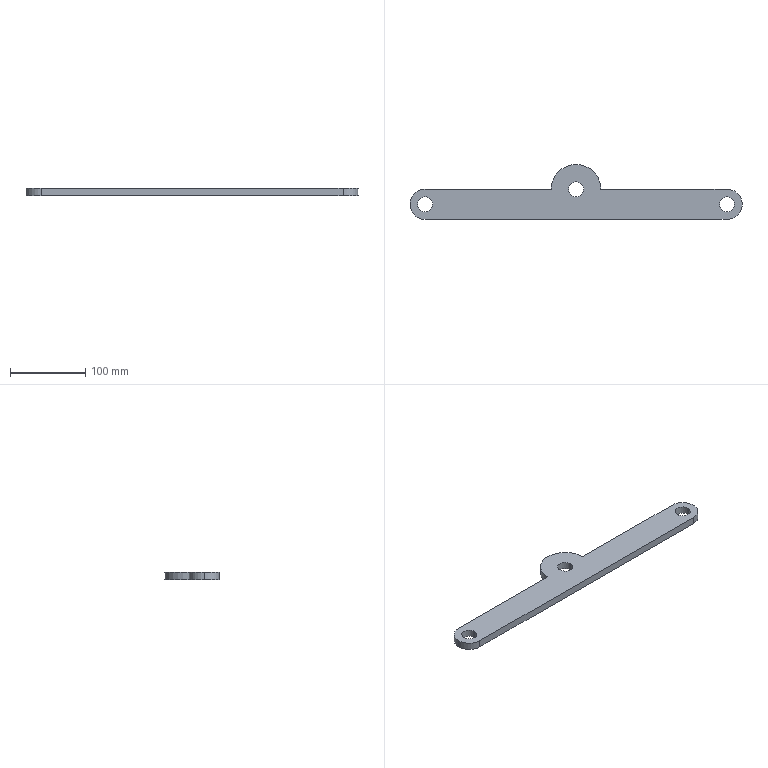Part | SolidWorks | features ICE 3, Extrusion 1 | 1 solid | 15 faces | box 440 x 72.879 x 10 mm | volume 180122 mm3 | cylinder 10 | plane 5 | commonest cylinder face diameters 20 x6 40 x3 65.758 x1
STEP:
#1=CARTESIAN_POINT('',(-10.,20.,0.));
#2=VERTEX_POINT('',#1);
#3=CARTESIAN_POINT('',(10.,20.,0.));
#4=VERTEX_POINT('',#3);
#5=CARTESIAN_POINT('',(0.,20.,0.));
#6=DIRECTION('',(0.,0.,1.));
#7=DIRECTION('',(1.,0.,0.));
#8=AXIS2_PLACEMENT_3D('',#5,#6,#7);
#9=CIRCLE('',#8,10.);
#10=EDGE_CURVE('',#2,#4,#9,.T.);
#11=ORIENTED_EDGE('',*,*,#10,.F.);
#12=CARTESIAN_POINT('',(-10.,20.,10.));
#13=VERTEX_POINT('',#12);
#14=CARTESIAN_POINT('',(-10.,20.,0.));
#15=DIRECTION('',(0.,0.,1.));
#16=VECTOR('',#15,1000.);
#17=LINE('',#14,#16);
#18=EDGE_CURVE('',#2,#13,#17,.T.);
#19=ORIENTED_EDGE('',*,*,#18,.T.);
#20=CARTESIAN_POINT('',(10.,20.,10.));
#21=VERTEX_POINT('',#20);
#22=CARTESIAN_POINT('',(0.,20.,10.));
#23=DIRECTION('',(0.,0.,1.));
#24=DIRECTION('',(1.,0.,0.));
#25=AXIS2_PLACEMENT_3D('',#22,#23,#24);
#26=CIRCLE('',#25,10.);
#27=EDGE_CURVE('',#13,#21,#26,.T.);
#28=ORIENTED_EDGE('',*,*,#27,.T.);
#29=CARTESIAN_POINT('',(10.,20.,0.));
#30=DIRECTION('',(0.,0.,1.));
#31=VECTOR('',#30,1000.);
#32=LINE('',#29,#31);
#33=EDGE_CURVE('',#4,#21,#32,.T.);
#34=ORIENTED_EDGE('',*,*,#33,.F.);
#35=EDGE_LOOP('',(#11,#19,#28,#34));
#36=FACE_OUTER_BOUND('',#35,.T.);
#37=CARTESIAN_POINT('',(0.,20.,0.));
#38=DIRECTION('',(0.,0.,1.));
#39=DIRECTION('',(1.,0.,0.));
#40=AXIS2_PLACEMENT_3D('',#37,#38,#39);
#41=CYLINDRICAL_SURFACE('',#40,10.);
#42=ADVANCED_FACE('',(#36),#41,.F.);
#43=CARTESIAN_POINT('',(-210.,0.,0.));
#44=VERTEX_POINT('',#43);
#45=CARTESIAN_POINT('',(-190.,0.,0.));
#46=VERTEX_POINT('',#45);
#47=CARTESIAN_POINT('',(-200.,0.,0.));
#48=DIRECTION('',(0.,0.,1.));
#49=DIRECTION('',(1.,0.,0.));
#50=AXIS2_PLACEMENT_3D('',#47,#48,#49);
#51=CIRCLE('',#50,10.);
#52=EDGE_CURVE('',#44,#46,#51,.T.);
#53=ORIENTED_EDGE('',*,*,#52,.F.);
#54=CARTESIAN_POINT('',(-210.,0.,10.));
#55=VERTEX_POINT('',#54);
#56=CARTESIAN_POINT('',(-210.,0.,0.));
#57=DIRECTION('',(0.,0.,1.));
#58=VECTOR('',#57,1000.);
#59=LINE('',#56,#58);
#60=EDGE_CURVE('',#44,#55,#59,.T.);
#61=ORIENTED_EDGE('',*,*,#60,.T.);
#62=CARTESIAN_POINT('',(-190.,0.,10.));
#63=VERTEX_POINT('',#62);
#64=CARTESIAN_POINT('',(-200.,0.,10.));
#65=DIRECTION('',(0.,0.,1.));
#66=DIRECTION('',(1.,0.,0.));
#67=AXIS2_PLACEMENT_3D('',#64,#65,#66);
#68=CIRCLE('',#67,10.);
#69=EDGE_CURVE('',#55,#63,#68,.T.);
#70=ORIENTED_EDGE('',*,*,#69,.T.);
#71=CARTESIAN_POINT('',(-190.,0.,0.));
#72=DIRECTION('',(0.,0.,1.));
#73=VECTOR('',#72,1000.);
#74=LINE('',#71,#73);
#75=EDGE_CURVE('',#46,#63,#74,.T.);
#76=ORIENTED_EDGE('',*,*,#75,.F.);
#77=EDGE_LOOP('',(#53,#61,#70,#76));
#78=FACE_OUTER_BOUND('',#77,.T.);
#79=CARTESIAN_POINT('',(-200.,0.,0.));
#80=DIRECTION('',(0.,0.,1.));
#81=DIRECTION('',(1.,0.,0.));
#82=AXIS2_PLACEMENT_3D('',#79,#80,#81);
#83=CYLINDRICAL_SURFACE('',#82,10.);
#84=ADVANCED_FACE('',(#78),#83,.F.);
#85=CARTESIAN_POINT('',(190.,0.,0.));
#86=VERTEX_POINT('',#85);
#87=CARTESIAN_POINT('',(210.,0.,0.));
#88=VERTEX_POINT('',#87);
#89=CARTESIAN_POINT('',(200.,0.,0.));
#90=DIRECTION('',(0.,0.,1.));
#91=DIRECTION('',(1.,0.,0.));
#92=AXIS2_PLACEMENT_3D('',#89,#90,#91);
#93=CIRCLE('',#92,10.);
#94=EDGE_CURVE('',#86,#88,#93,.T.);
#95=ORIENTED_EDGE('',*,*,#94,.F.);
#96=CARTESIAN_POINT('',(190.,0.,10.));
#97=VERTEX_POINT('',#96);
#98=CARTESIAN_POINT('',(190.,0.,0.));
#99=DIRECTION('',(0.,0.,1.));
#100=VECTOR('',#99,1000.);
#101=LINE('',#98,#100);
#102=EDGE_CURVE('',#86,#97,#101,.T.);
#103=ORIENTED_EDGE('',*,*,#102,.T.);
#104=CARTESIAN_POINT('',(210.,0.,10.));
#105=VERTEX_POINT('',#104);
#106=CARTESIAN_POINT('',(200.,0.,10.));
#107=DIRECTION('',(0.,0.,1.));
#108=DIRECTION('',(1.,0.,0.));
#109=AXIS2_PLACEMENT_3D('',#106,#107,#108);
#110=CIRCLE('',#109,10.);
#111=EDGE_CURVE('',#97,#105,#110,.T.);
#112=ORIENTED_EDGE('',*,*,#111,.T.);
#113=CARTESIAN_POINT('',(210.,0.,0.));
#114=DIRECTION('',(0.,0.,1.));
#115=VECTOR('',#114,1000.);
#116=LINE('',#113,#115);
#117=EDGE_CURVE('',#88,#105,#116,.T.);
#118=ORIENTED_EDGE('',*,*,#117,.F.);
#119=EDGE_LOOP('',(#95,#103,#112,#118));
#120=FACE_OUTER_BOUND('',#119,.T.);
#121=CARTESIAN_POINT('',(200.,0.,0.));
#122=DIRECTION('',(0.,0.,1.));
#123=DIRECTION('',(1.,0.,0.));
#124=AXIS2_PLACEMENT_3D('',#121,#122,#123);
#125=CYLINDRICAL_SURFACE('',#124,10.);
#126=ADVANCED_FACE('',(#120),#125,.F.);
#127=CARTESIAN_POINT('',(-220.,0.,10.));
#128=VERTEX_POINT('',#127);
#129=CARTESIAN_POINT('',(-200.,-20.,10.));
#130=VERTEX_POINT('',#129);
#131=CARTESIAN_POINT('',(-200.,0.,10.));
#132=DIRECTION('',(0.,0.,1.));
#133=DIRECTION('',(1.,0.,0.));
#134=AXIS2_PLACEMENT_3D('',#131,#132,#133);
#135=CIRCLE('',#134,20.);
#136=EDGE_CURVE('',#128,#130,#135,.T.);
#137=ORIENTED_EDGE('',*,*,#136,.F.);
#138=CARTESIAN_POINT('',(-220.,0.,0.));
#139=VERTEX_POINT('',#138);
#140=CARTESIAN_POINT('',(-220.,0.,10.));
#141=DIRECTION('',(0.,0.,-1.));
#142=VECTOR('',#141,1000.);
#143=LINE('',#140,#142);
#144=EDGE_CURVE('',#128,#139,#143,.T.);
#145=ORIENTED_EDGE('',*,*,#144,.T.);
#146=CARTESIAN_POINT('',(-200.,-20.,0.));
#147=VERTEX_POINT('',#146);
#148=CARTESIAN_POINT('',(-200.,0.,0.));
#149=DIRECTION('',(0.,0.,1.));
#150=DIRECTION('',(1.,0.,0.));
#151=AXIS2_PLACEMENT_3D('',#148,#149,#150);
#152=CIRCLE('',#151,20.);
#153=EDGE_CURVE('',#139,#147,#152,.T.);
#154=ORIENTED_EDGE('',*,*,#153,.T.);
#155=CARTESIAN_POINT('',(-200.,-20.,10.));
#156=DIRECTION('',(0.,0.,-1.));
#157=VECTOR('',#156,1000.);
#158=LINE('',#155,#157);
#159=EDGE_CURVE('',#130,#147,#158,.T.);
#160=ORIENTED_EDGE('',*,*,#159,.F.);
#161=EDGE_LOOP('',(#137,#145,#154,#160));
#162=FACE_OUTER_BOUND('',#161,.T.);
#163=CARTESIAN_POINT('',(-200.,0.,10.));
#164=DIRECTION('',(0.,0.,-1.));
#165=DIRECTION('',(-1.,0.,0.));
#166=AXIS2_PLACEMENT_3D('',#163,#164,#165);
#167=CYLINDRICAL_SURFACE('',#166,20.);
#168=ADVANCED_FACE('',(#162),#167,.T.);
#169=CARTESIAN_POINT('',(200.,20.,0.));
#170=VERTEX_POINT('',#169);
#171=CARTESIAN_POINT('',(32.879,20.,0.));
#172=VERTEX_POINT('',#171);
#173=CARTESIAN_POINT('',(-200.,20.,0.));
#174=DIRECTION('',(-1.,0.,0.));
#175=VECTOR('',#174,1000.);
#176=LINE('',#173,#175);
#177=EDGE_CURVE('',#170,#172,#176,.T.);
#178=ORIENTED_EDGE('',*,*,#177,.T.);
#179=CARTESIAN_POINT('',(32.879,20.,10.));
#180=VERTEX_POINT('',#179);
#181=CARTESIAN_POINT('',(32.879,20.,-92.996));
#182=DIRECTION('',(0.,0.,1.));
#183=VECTOR('',#182,1000.);
#184=LINE('',#181,#183);
#185=EDGE_CURVE('',#172,#180,#184,.T.);
#186=ORIENTED_EDGE('',*,*,#185,.T.);
#187=CARTESIAN_POINT('',(200.,20.,10.));
#188=VERTEX_POINT('',#187);
#189=CARTESIAN_POINT('',(-200.,20.,10.));
#190=DIRECTION('',(-1.,0.,0.));
#191=VECTOR('',#190,1000.);
#192=LINE('',#189,#191);
#193=EDGE_CURVE('',#188,#180,#192,.T.);
#194=ORIENTED_EDGE('',*,*,#193,.F.);
#195=CARTESIAN_POINT('',(200.,20.,10.));
#196=DIRECTION('',(0.,0.,-1.));
#197=VECTOR('',#196,1000.);
#198=LINE('',#195,#197);
#199=EDGE_CURVE('',#188,#170,#198,.T.);
#200=ORIENTED_EDGE('',*,*,#199,.T.);
#201=EDGE_LOOP('',(#178,#186,#194,#200));
#202=FACE_OUTER_BOUND('',#201,.T.);
#203=CARTESIAN_POINT('',(-200.,20.,10.));
#204=DIRECTION('',(0.,-1.,0.));
#205=DIRECTION('',(1.,0.,0.));
#206=AXIS2_PLACEMENT_3D('',#203,#204,#205);
#207=PLANE('',#206);
#208=ADVANCED_FACE('',(#202),#207,.F.);
#209=ORIENTED_EDGE('',*,*,#144,.F.);
#210=CARTESIAN_POINT('',(-200.,20.,10.));
#211=VERTEX_POINT('',#210);
#212=CARTESIAN_POINT('',(-200.,0.,10.));
#213=DIRECTION('',(0.,0.,1.));
#214=DIRECTION('',(1.,0.,0.));
#215=AXIS2_PLACEMENT_3D('',#212,#213,#214);
#216=CIRCLE('',#215,20.);
#217=EDGE_CURVE('',#211,#128,#216,.T.);
#218=ORIENTED_EDGE('',*,*,#217,.F.);
#219=CARTESIAN_POINT('',(-200.,20.,0.));
#220=VERTEX_POINT('',#219);
#221=CARTESIAN_POINT('',(-200.,20.,10.));
#222=DIRECTION('',(0.,0.,-1.));
#223=VECTOR('',#222,1000.);
#224=LINE('',#221,#223);
#225=EDGE_CURVE('',#211,#220,#224,.T.);
#226=ORIENTED_EDGE('',*,*,#225,.T.);
#227=CARTESIAN_POINT('',(-200.,0.,0.));
#228=DIRECTION('',(0.,0.,1.));
#229=DIRECTION('',(1.,0.,0.));
#230=AXIS2_PLACEMENT_3D('',#227,#228,#229);
#231=CIRCLE('',#230,20.);
#232=EDGE_CURVE('',#220,#139,#231,.T.);
#233=ORIENTED_EDGE('',*,*,#232,.T.);
#234=EDGE_LOOP('',(#209,#218,#226,#233));
#235=FACE_OUTER_BOUND('',#234,.T.);
#236=CARTESIAN_POINT('',(-200.,0.,10.));
#237=DIRECTION('',(0.,0.,-1.));
#238=DIRECTION('',(-1.,0.,0.));
#239=AXIS2_PLACEMENT_3D('',#236,#237,#238);
#240=CYLINDRICAL_SURFACE('',#239,20.);
#241=ADVANCED_FACE('',(#235),#240,.T.);
#242=CARTESIAN_POINT('',(200.,-20.,0.));
#243=VERTEX_POINT('',#242);
#244=CARTESIAN_POINT('',(-200.,-20.,0.));
#245=DIRECTION('',(1.,0.,0.));
#246=VECTOR('',#245,1000.);
#247=LINE('',#244,#246);
#248=EDGE_CURVE('',#147,#243,#247,.T.);
#249=ORIENTED_EDGE('',*,*,#248,.T.);
#250=CARTESIAN_POINT('',(200.,-20.,10.));
#251=VERTEX_POINT('',#250);
#252=CARTESIAN_POINT('',(200.,-20.,10.));
#253=DIRECTION('',(0.,0.,-1.));
#254=VECTOR('',#253,1000.);
#255=LINE('',#252,#254);
#256=EDGE_CURVE('',#251,#243,#255,.T.);
#257=ORIENTED_EDGE('',*,*,#256,.F.);
#258=CARTESIAN_POINT('',(-200.,-20.,10.));
#259=DIRECTION('',(1.,0.,0.));
#260=VECTOR('',#259,1000.);
#261=LINE('',#258,#260);
#262=EDGE_CURVE('',#130,#251,#261,.T.);
#263=ORIENTED_EDGE('',*,*,#262,.F.);
#264=ORIENTED_EDGE('',*,*,#159,.T.);
#265=EDGE_LOOP('',(#249,#257,#263,#264));
#266=FACE_OUTER_BOUND('',#265,.T.);
#267=CARTESIAN_POINT('',(-200.,-20.,10.));
#268=DIRECTION('',(0.,1.,0.));
#269=DIRECTION('',(0.,0.,1.));
#270=AXIS2_PLACEMENT_3D('',#267,#268,#269);
#271=PLANE('',#270);
#272=ADVANCED_FACE('',(#266),#271,.F.);
#273=CARTESIAN_POINT('',(200.,0.,0.));
#274=DIRECTION('',(0.,0.,1.));
#275=DIRECTION('',(1.,0.,0.));
#276=AXIS2_PLACEMENT_3D('',#273,#274,#275);
#277=CIRCLE('',#276,20.);
#278=EDGE_CURVE('',#243,#170,#277,.T.);
#279=ORIENTED_EDGE('',*,*,#278,.T.);
#280=ORIENTED_EDGE('',*,*,#199,.F.);
#281=CARTESIAN_POINT('',(200.,0.,10.));
#282=DIRECTION('',(0.,0.,1.));
#283=DIRECTION('',(1.,0.,0.));
#284=AXIS2_PLACEMENT_3D('',#281,#282,#283);
#285=CIRCLE('',#284,20.);
#286=EDGE_CURVE('',#251,#188,#285,.T.);
#287=ORIENTED_EDGE('',*,*,#286,.F.);
#288=ORIENTED_EDGE('',*,*,#256,.T.);
#289=EDGE_LOOP('',(#279,#280,#287,#288));
#290=FACE_OUTER_BOUND('',#289,.T.);
#291=CARTESIAN_POINT('',(200.,0.,10.));
#292=DIRECTION('',(0.,0.,-1.));
#293=DIRECTION('',(-1.,0.,0.));
#294=AXIS2_PLACEMENT_3D('',#291,#292,#293);
#295=CYLINDRICAL_SURFACE('',#294,20.);
#296=ADVANCED_FACE('',(#290),#295,.T.);
#297=CARTESIAN_POINT('',(-32.879,20.,10.));
#298=VERTEX_POINT('',#297);
#299=CARTESIAN_POINT('',(-200.,20.,10.));
#300=DIRECTION('',(-1.,0.,0.));
#301=VECTOR('',#300,1000.);
#302=LINE('',#299,#301);
#303=EDGE_CURVE('',#298,#211,#302,.T.);
#304=ORIENTED_EDGE('',*,*,#303,.F.);
#305=CARTESIAN_POINT('',(-32.879,20.,0.));
#306=VERTEX_POINT('',#305);
#307=CARTESIAN_POINT('',(-32.879,20.,-92.996));
#308=DIRECTION('',(0.,0.,-1.));
#309=VECTOR('',#308,1000.);
#310=LINE('',#307,#309);
#311=EDGE_CURVE('',#298,#306,#310,.T.);
#312=ORIENTED_EDGE('',*,*,#311,.T.);
#313=CARTESIAN_POINT('',(-200.,20.,0.));
#314=DIRECTION('',(-1.,0.,0.));
#315=VECTOR('',#314,1000.);
#316=LINE('',#313,#315);
#317=EDGE_CURVE('',#306,#220,#316,.T.);
#318=ORIENTED_EDGE('',*,*,#317,.T.);
#319=ORIENTED_EDGE('',*,*,#225,.F.);
#320=EDGE_LOOP('',(#304,#312,#318,#319));
#321=FACE_OUTER_BOUND('',#320,.T.);
#322=CARTESIAN_POINT('',(-200.,20.,10.));
#323=DIRECTION('',(0.,-1.,0.));
#324=DIRECTION('',(1.,0.,0.));
#325=AXIS2_PLACEMENT_3D('',#322,#323,#324);
#326=PLANE('',#325);
#327=ADVANCED_FACE('',(#321),#326,.F.);
#328=CARTESIAN_POINT('',(0.,20.,10.));
#329=DIRECTION('',(0.,0.,1.));
#330=DIRECTION('',(1.,0.,0.));
#331=AXIS2_PLACEMENT_3D('',#328,#329,#330);
#332=CIRCLE('',#331,10.);
#333=EDGE_CURVE('',#21,#13,#332,.T.);
#334=ORIENTED_EDGE('',*,*,#333,.F.);
#335=ORIENTED_EDGE('',*,*,#27,.F.);
#336=EDGE_LOOP('',(#334,#335));
#337=FACE_BOUND('',#336,.T.);
#338=ORIENTED_EDGE('',*,*,#193,.T.);
#339=CARTESIAN_POINT('',(0.,20.,10.));
#340=DIRECTION('',(0.,0.,1.));
#341=DIRECTION('',(1.,0.,0.));
#342=AXIS2_PLACEMENT_3D('',#339,#340,#341);
#343=CIRCLE('',#342,32.879);
#344=EDGE_CURVE('',#180,#298,#343,.T.);
#345=ORIENTED_EDGE('',*,*,#344,.T.);
#346=ORIENTED_EDGE('',*,*,#303,.T.);
#347=ORIENTED_EDGE('',*,*,#217,.T.);
#348=ORIENTED_EDGE('',*,*,#136,.T.);
#349=ORIENTED_EDGE('',*,*,#262,.T.);
#350=ORIENTED_EDGE('',*,*,#286,.T.);
#351=EDGE_LOOP('',(#338,#345,#346,#347,#348,#349,#350));
#352=FACE_OUTER_BOUND('',#351,.T.);
#353=CARTESIAN_POINT('',(-200.,0.,10.));
#354=DIRECTION('',(0.,0.,1.));
#355=DIRECTION('',(1.,0.,0.));
#356=AXIS2_PLACEMENT_3D('',#353,#354,#355);
#357=CIRCLE('',#356,10.);
#358=EDGE_CURVE('',#63,#55,#357,.T.);
#359=ORIENTED_EDGE('',*,*,#358,.F.);
#360=ORIENTED_EDGE('',*,*,#69,.F.);
#361=EDGE_LOOP('',(#359,#360));
#362=FACE_BOUND('',#361,.T.);
#363=CARTESIAN_POINT('',(200.,0.,10.));
#364=DIRECTION('',(0.,0.,1.));
#365=DIRECTION('',(1.,0.,0.));
#366=AXIS2_PLACEMENT_3D('',#363,#364,#365);
#367=CIRCLE('',#366,10.);
#368=EDGE_CURVE('',#105,#97,#367,.T.);
#369=ORIENTED_EDGE('',*,*,#368,.F.);
#370=ORIENTED_EDGE('',*,*,#111,.F.);
#371=EDGE_LOOP('',(#369,#370));
#372=FACE_BOUND('',#371,.T.);
#373=CARTESIAN_POINT('',(-200.,0.,10.));
#374=DIRECTION('',(0.,0.,1.));
#375=DIRECTION('',(1.,0.,0.));
#376=AXIS2_PLACEMENT_3D('',#373,#374,#375);
#377=PLANE('',#376);
#378=ADVANCED_FACE('',(#337,#352,#362,#372),#377,.T.);
#379=CARTESIAN_POINT('',(0.,20.,0.));
#380=DIRECTION('',(0.,0.,1.));
#381=DIRECTION('',(1.,0.,0.));
#382=AXIS2_PLACEMENT_3D('',#379,#380,#381);
#383=CIRCLE('',#382,10.);
#384=EDGE_CURVE('',#4,#2,#383,.T.);
#385=ORIENTED_EDGE('',*,*,#384,.T.);
#386=ORIENTED_EDGE('',*,*,#10,.T.);
#387=EDGE_LOOP('',(#385,#386));
#388=FACE_BOUND('',#387,.T.);
#389=CARTESIAN_POINT('',(-200.,0.,0.));
#390=DIRECTION('',(0.,0.,1.));
#391=DIRECTION('',(1.,0.,0.));
#392=AXIS2_PLACEMENT_3D('',#389,#390,#391);
#393=CIRCLE('',#392,10.);
#394=EDGE_CURVE('',#46,#44,#393,.T.);
#395=ORIENTED_EDGE('',*,*,#394,.T.);
#396=ORIENTED_EDGE('',*,*,#52,.T.);
#397=EDGE_LOOP('',(#395,#396));
#398=FACE_BOUND('',#397,.T.);
#399=CARTESIAN_POINT('',(200.,0.,0.));
#400=DIRECTION('',(0.,0.,1.));
#401=DIRECTION('',(1.,0.,0.));
#402=AXIS2_PLACEMENT_3D('',#399,#400,#401);
#403=CIRCLE('',#402,10.);
#404=EDGE_CURVE('',#88,#86,#403,.T.);
#405=ORIENTED_EDGE('',*,*,#404,.T.);
#406=ORIENTED_EDGE('',*,*,#94,.T.);
#407=EDGE_LOOP('',(#405,#406));
#408=FACE_BOUND('',#407,.T.);
#409=ORIENTED_EDGE('',*,*,#317,.F.);
#410=CARTESIAN_POINT('',(0.,20.,0.));
#411=DIRECTION('',(0.,0.,-1.));
#412=DIRECTION('',(1.,0.,0.));
#413=AXIS2_PLACEMENT_3D('',#410,#411,#412);
#414=CIRCLE('',#413,32.879);
#415=EDGE_CURVE('',#306,#172,#414,.T.);
#416=ORIENTED_EDGE('',*,*,#415,.T.);
#417=ORIENTED_EDGE('',*,*,#177,.F.);
#418=ORIENTED_EDGE('',*,*,#278,.F.);
#419=ORIENTED_EDGE('',*,*,#248,.F.);
#420=ORIENTED_EDGE('',*,*,#153,.F.);
#421=ORIENTED_EDGE('',*,*,#232,.F.);
#422=EDGE_LOOP('',(#409,#416,#417,#418,#419,#420,#421));
#423=FACE_OUTER_BOUND('',#422,.T.);
#424=CARTESIAN_POINT('',(-200.,0.,0.));
#425=DIRECTION('',(0.,0.,1.));
#426=DIRECTION('',(1.,0.,0.));
#427=AXIS2_PLACEMENT_3D('',#424,#425,#426);
#428=PLANE('',#427);
#429=ADVANCED_FACE('',(#388,#398,#408,#423),#428,.F.);
#430=ORIENTED_EDGE('',*,*,#102,.F.);
#431=ORIENTED_EDGE('',*,*,#404,.F.);
#432=ORIENTED_EDGE('',*,*,#117,.T.);
#433=ORIENTED_EDGE('',*,*,#368,.T.);
#434=EDGE_LOOP('',(#430,#431,#432,#433));
#435=FACE_OUTER_BOUND('',#434,.T.);
#436=CARTESIAN_POINT('',(200.,0.,0.));
#437=DIRECTION('',(0.,0.,1.));
#438=DIRECTION('',(1.,0.,0.));
#439=AXIS2_PLACEMENT_3D('',#436,#437,#438);
#440=CYLINDRICAL_SURFACE('',#439,10.);
#441=ADVANCED_FACE('',(#435),#440,.F.);
#442=ORIENTED_EDGE('',*,*,#60,.F.);
#443=ORIENTED_EDGE('',*,*,#394,.F.);
#444=ORIENTED_EDGE('',*,*,#75,.T.);
#445=ORIENTED_EDGE('',*,*,#358,.T.);
#446=EDGE_LOOP('',(#442,#443,#444,#445));
#447=FACE_OUTER_BOUND('',#446,.T.);
#448=CARTESIAN_POINT('',(-200.,0.,0.));
#449=DIRECTION('',(0.,0.,1.));
#450=DIRECTION('',(1.,0.,0.));
#451=AXIS2_PLACEMENT_3D('',#448,#449,#450);
#452=CYLINDRICAL_SURFACE('',#451,10.);
#453=ADVANCED_FACE('',(#447),#452,.F.);
#454=ORIENTED_EDGE('',*,*,#185,.F.);
#455=ORIENTED_EDGE('',*,*,#415,.F.);
#456=ORIENTED_EDGE('',*,*,#311,.F.);
#457=ORIENTED_EDGE('',*,*,#344,.F.);
#458=EDGE_LOOP('',(#454,#455,#456,#457));
#459=FACE_OUTER_BOUND('',#458,.T.);
#460=CARTESIAN_POINT('',(0.,20.,-92.996));
#461=DIRECTION('',(0.,0.,1.));
#462=DIRECTION('',(1.,0.,0.));
#463=AXIS2_PLACEMENT_3D('',#460,#461,#462);
#464=CYLINDRICAL_SURFACE('',#463,32.879);
#465=ADVANCED_FACE('',(#459),#464,.T.);
#466=ORIENTED_EDGE('',*,*,#18,.F.);
#467=ORIENTED_EDGE('',*,*,#384,.F.);
#468=ORIENTED_EDGE('',*,*,#33,.T.);
#469=ORIENTED_EDGE('',*,*,#333,.T.);
#470=EDGE_LOOP('',(#466,#467,#468,#469));
#471=FACE_OUTER_BOUND('',#470,.T.);
#472=CARTESIAN_POINT('',(0.,20.,0.));
#473=DIRECTION('',(0.,0.,1.));
#474=DIRECTION('',(1.,0.,0.));
#475=AXIS2_PLACEMENT_3D('',#472,#473,#474);
#476=CYLINDRICAL_SURFACE('',#475,10.);
#477=ADVANCED_FACE('',(#471),#476,.F.);
#478=CLOSED_SHELL('',(#42,#84,#126,#168,#208,#241,#272,#296,#327,#378,#429,#441,#453,#465,#477));
#479=MANIFOLD_SOLID_BREP('',#478);
#480=CARTESIAN_POINT('',(0.,0.,0.));
#481=DIRECTION('',(0.,0.,1.));
#482=DIRECTION('',(1.,0.,0.));
#483=AXIS2_PLACEMENT_3D('',#480,#481,#482);
#484=(LENGTH_UNIT()NAMED_UNIT(*)SI_UNIT(.MILLI.,.METRE.));
#485=UNCERTAINTY_MEASURE_WITH_UNIT(LENGTH_MEASURE(0.00001),#484,'','');
#486=(NAMED_UNIT(*)PLANE_ANGLE_UNIT()SI_UNIT($,.RADIAN.));
#487=(NAMED_UNIT(*)SI_UNIT($,.STERADIAN.)SOLID_ANGLE_UNIT());
#488=(GEOMETRIC_REPRESENTATION_CONTEXT(3)GLOBAL_UNCERTAINTY_ASSIGNED_CONTEXT((#485))GLOBAL_UNIT_ASSIGNED_CONTEXT((#484,#486,#487))REPRESENTATION_CONTEXT('',''));
#489=ADVANCED_BREP_SHAPE_REPRESENTATION('',(#479,#483),#488);